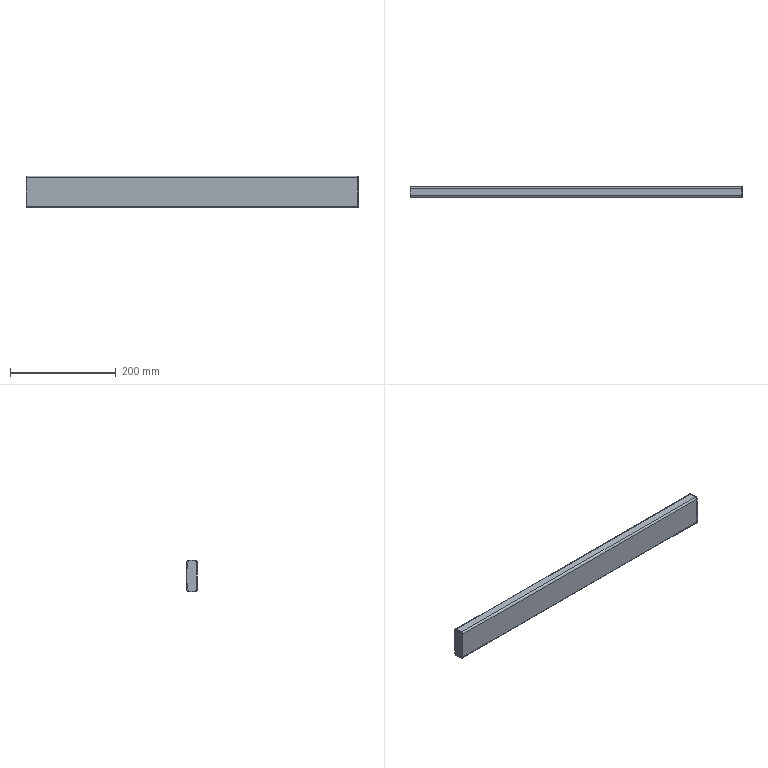Part | SolidWorks | features FlatPattern 4, EdgeFlange 2, SMBaseFlange 2, SheetMetal 2, HoleWzd 1, ICE 1, LPattern 1, MirrorSolid 1 | 6 solids | 82 faces | box 628 x 20 x 60 mm | volume 120616 mm3 | plane 60 | cylinder 22 | commonest cylinder face diameters 7 x12 5 x6 4 x4